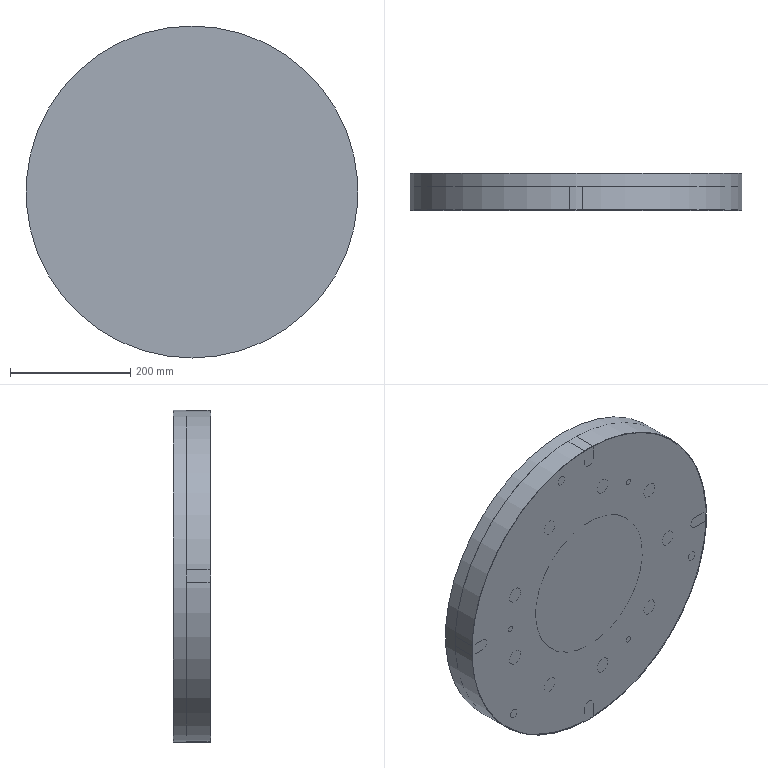NC program | NX | posted with a generic post | part box 552 x 62 x 552 mm
Whole program:
N10 G17 G21 G94 G90
(铣键槽 , TOOL : D8)
N12 T03 M6
N14 G54
N16 G17 G0 G90 X161.06 Y-135.798 S2666 M3
N18 G43 Z19. H3
N20 Z-20.
N22 G94 G1 X168.726 Y-142.231 Z-20.262 F90.
N24 X169.005 Y-142.257 Z-20.269
N26 X169.258 Y-142.137 Z-20.277
N28 X169.434 Y-141.832 Z-20.286
N30 X169.369 Y-141.465 Z-20.296
N32 X160.673 Y-134.168 Z-20.593
N34 X160.394 Y-134.142 Z-20.6
N36 X160.141 Y-134.262 Z-20.608
N38 X159.965 Y-134.566 Z-20.617
N40 X160.03 Y-134.934 Z-20.627
N42 X168.726 Y-142.231 Z-20.924
N44 X169.005 Y-142.257 Z-20.931
N46 X169.258 Y-142.137 Z-20.939
N48 X169.434 Y-141.832 Z-20.948
N50 X169.369 Y-141.465 Z-20.958
N52 X160.673 Y-134.168 Z-21.255
N54 X160.394 Y-134.142 Z-21.262
N56 X160.141 Y-134.262 Z-21.269
N58 X159.965 Y-134.566 Z-21.279
N60 X160.03 Y-134.934 Z-21.288
N62 X168.726 Y-142.231 Z-21.586
N64 X169.005 Y-142.257 Z-21.593
N66 X169.258 Y-142.137 Z-21.6
N68 X169.434 Y-141.832 Z-21.61
N70 X169.369 Y-141.465 Z-21.619
N72 X160.673 Y-134.168 Z-21.917
N74 X160.394 Y-134.142 Z-21.924
N76 X160.141 Y-134.262 Z-21.931
N78 X159.965 Y-134.566 Z-21.94
N80 X160.03 Y-134.934 Z-21.95
N82 X168.726 Y-142.231 Z-22.247
N84 X169.005 Y-142.257 Z-22.255
N86 X169.258 Y-142.137 Z-22.262
N88 X169.434 Y-141.832 Z-22.271
N90 X169.369 Y-141.465 Z-22.281
N92 X169.234 Y-141.352 Z-22.286
N94 X160.808 Y-134.281
N96 G3 X160.103 Y-134.343 R0.5
N98 X160.165 Y-135.047 R0.5
N100 G1 X168.591 Y-142.118
N102 G3 X169.296 Y-142.056 R0.5
N104 X169.234 Y-141.352 R0.5
N106 G0 Z-21.7
N108 Z-22.571
N110 G1 X160.808 Y-134.281
N112 G3 X160.103 Y-134.343 R0.5
N114 X160.165 Y-135.047 R0.5
N116 G1 X168.591 Y-142.118
N118 G3 X169.296 Y-142.056 R0.5
N120 X169.234 Y-141.352 R0.5
N122 G0 Z-21.986
N124 Z-22.857
N126 G1 X160.808 Y-134.281
N128 G3 X160.103 Y-134.343 R0.5
N130 X160.165 Y-135.047 R0.5
N132 G1 X168.591 Y-142.118
N134 G3 X169.296 Y-142.056 R0.5
N136 X169.234 Y-141.352 R0.5
N138 G0 Z-22.271
N140 Z-23.143
N142 G1 X160.808 Y-134.281
N144 G3 X160.103 Y-134.343 R0.5
N146 X160.165 Y-135.047 R0.5
N148 G1 X168.591 Y-142.118
N150 G3 X169.296 Y-142.056 R0.5
N152 X169.234 Y-141.352 R0.5
N154 G0 Z-22.557
N156 Z-23.429
N158 G1 X160.808 Y-134.281
N160 G3 X160.103 Y-134.343 R0.5
N162 X160.165 Y-135.047 R0.5
N164 G1 X168.591 Y-142.118
N166 G3 X169.296 Y-142.056 R0.5
N168 X169.234 Y-141.352 R0.5
N170 G0 Z-22.843
N172 Z-23.714
N174 G1 X160.808 Y-134.281
N176 G3 X160.103 Y-134.343 R0.5
N178 X160.165 Y-135.047 R0.5
N180 G1 X168.591 Y-142.118
N182 G3 X169.296 Y-142.056 R0.5
N184 X169.234 Y-141.352 R0.5
N186 G0 Z-23.129
N188 Z-24.
N190 G1 X160.808 Y-134.281
N192 G3 X160.103 Y-134.343 R0.5
N194 X160.165 Y-135.047 R0.5
N196 G1 X168.591 Y-142.118
N198 G3 X169.296 Y-142.056 R0.5
N200 X169.234 Y-141.352 R0.5
N202 G0 Z-23.414
N204 Z-24.286
N206 G1 X160.808 Y-134.281
N208 G3 X160.103 Y-134.343 R0.5
N210 X160.165 Y-135.047 R0.5
N212 G1 X168.591 Y-142.118
N214 G3 X169.296 Y-142.056 R0.5
N216 X169.234 Y-141.352 R0.5
N218 G0 Z-23.7
N220 Z-24.571
N222 G1 X160.808 Y-134.281
N224 G3 X160.103 Y-134.343 R0.5
N226 X160.165 Y-135.047 R0.5
N228 G1 X168.591 Y-142.118
N230 G3 X169.296 Y-142.056 R0.5
N232 X169.234 Y-141.352 R0.5
N234 G0 Z-23.986
N236 Z-24.857
N238 G1 X160.808 Y-134.281
N240 G3 X160.103 Y-134.343 R0.5
N242 X160.165 Y-135.047 R0.5
N244 G1 X168.591 Y-142.118
N246 G3 X169.296 Y-142.056 R0.5
N248 X169.234 Y-141.352 R0.5
N250 G0 Z-24.271
N252 Z-25.143
N254 G1 X160.808 Y-134.281
N256 G3 X160.103 Y-134.343 R0.5
N258 X160.165 Y-135.047 R0.5
N260 G1 X168.591 Y-142.118
N262 G3 X169.296 Y-142.056 R0.5
N264 X169.234 Y-141.352 R0.5
N266 G0 Z-24.557
N268 Z-25.429
N270 G1 X160.808 Y-134.281
N272 G3 X160.103 Y-134.343 R0.5
N274 X160.165 Y-135.047 R0.5
N276 G1 X168.591 Y-142.118
N278 G3 X169.296 Y-142.056 R0.5
N280 X169.234 Y-141.352 R0.5
N282 G0 Z-24.843
N284 Z-25.714
N286 G1 X160.808 Y-134.281
N288 G3 X160.103 Y-134.343 R0.5
N290 X160.165 Y-135.047 R0.5
N292 G1 X168.591 Y-142.118
N294 G3 X169.296 Y-142.056 R0.5
N296 X169.234 Y-141.352 R0.5
N298 G0 Z-25.129
N300 Z-26.
N302 G1 X160.808 Y-134.281
N304 G3 X160.103 Y-134.343 R0.5
N306 X160.165 Y-135.047 R0.5
N308 G1 X168.591 Y-142.118
N310 G3 X169.296 Y-142.056 R0.5
N312 X169.234 Y-141.352 R0.5
N314 G1 Z-24.
N316 G0 Z19.
N318 M5
N320 M2